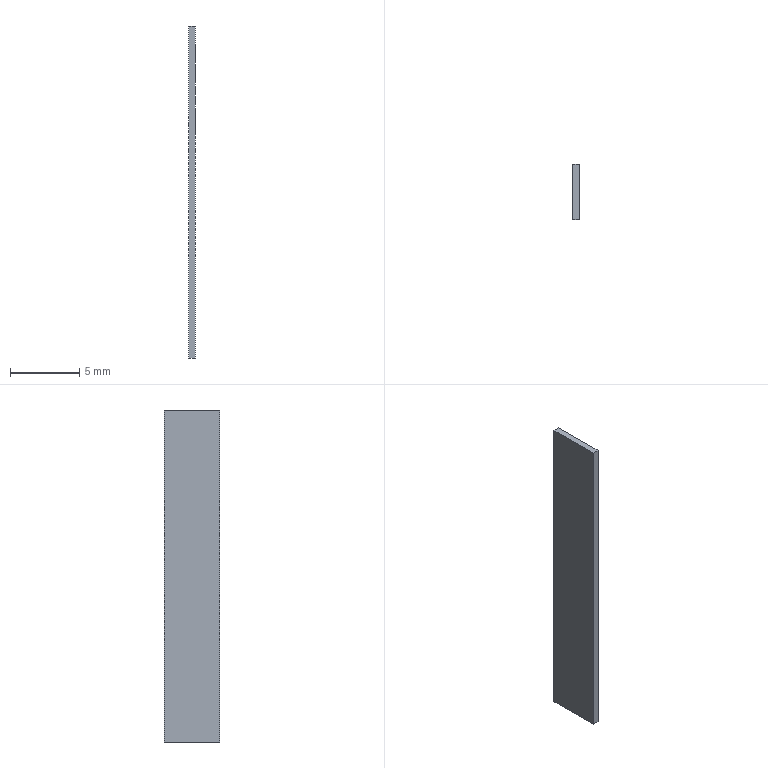Part | SolidWorks | features BaseBody 1 | 1 solid | 64 faces | box 0.5 x 4 x 24 mm | volume 47.328 mm3 | plane 37 | spline 27